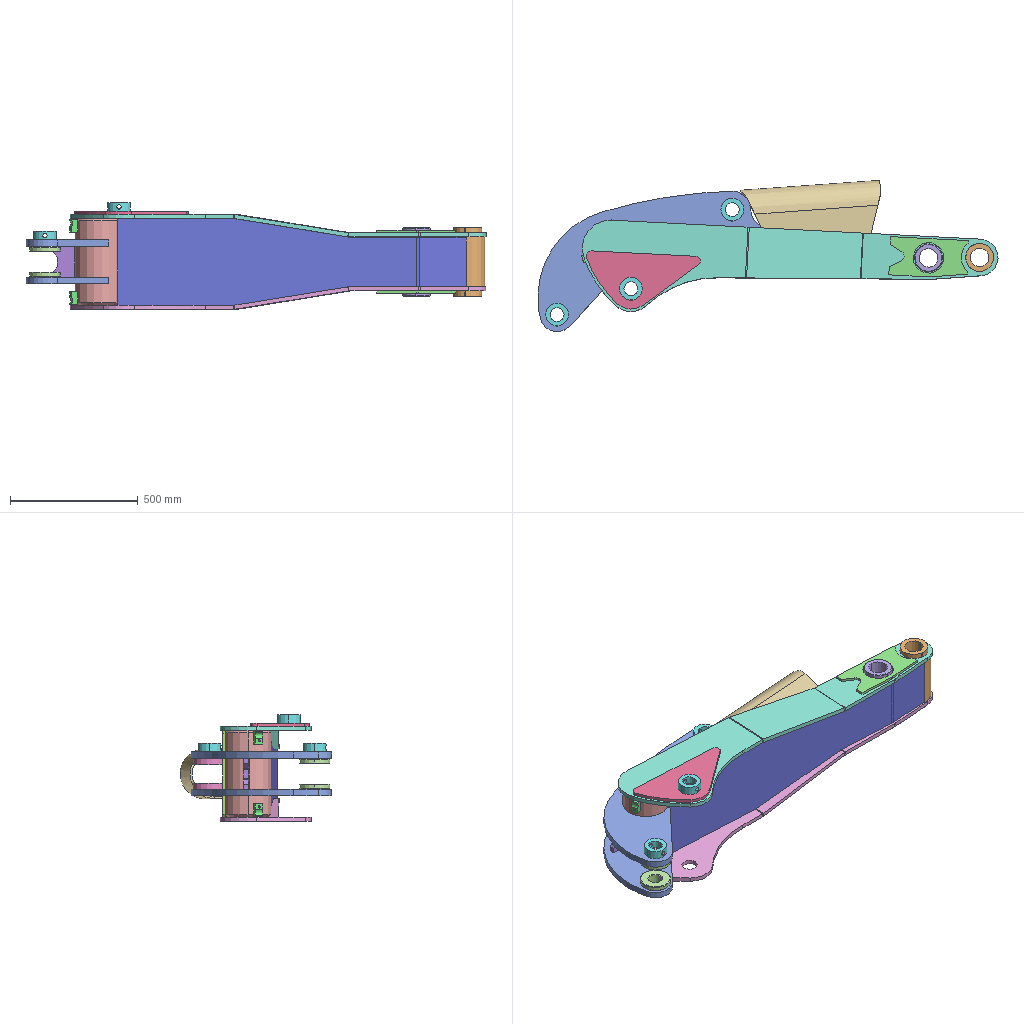Assembly | SolidWorks | 21 different items | 28 placed | box 1804 x 593 x 419 mm
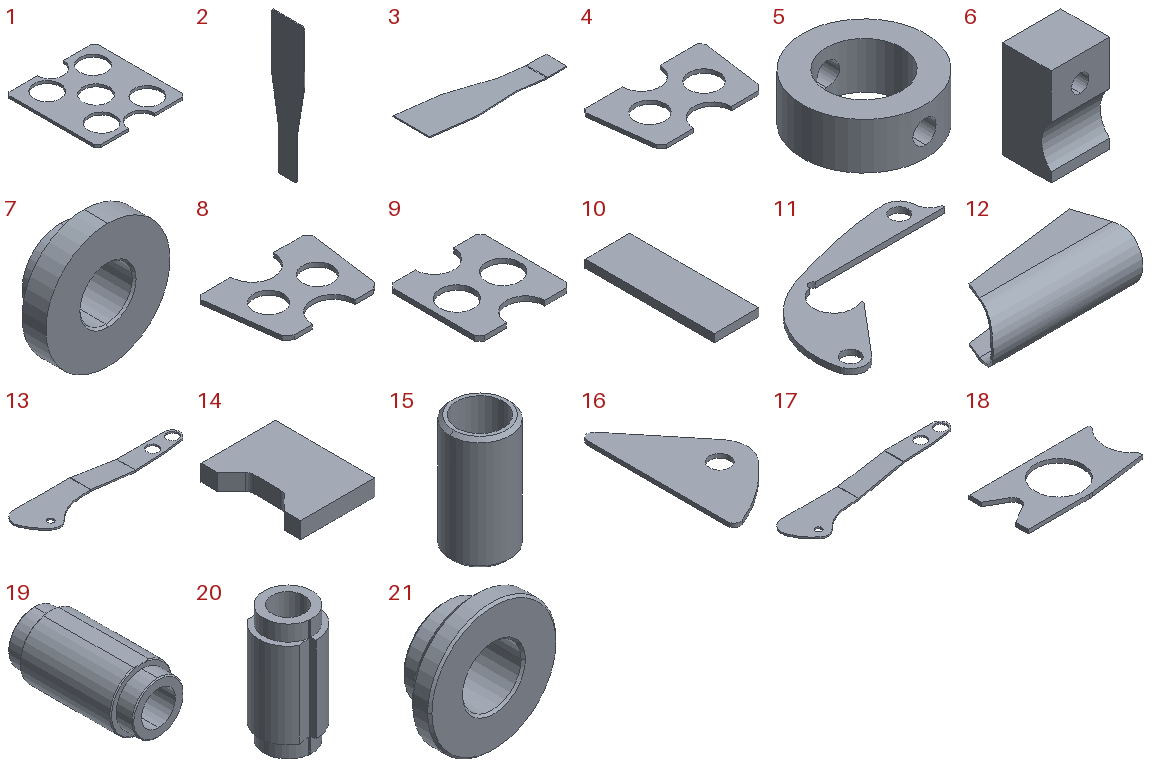Parts list (item | quantity | size | volume | features):
1 | x1 | 340 x 350 x 10 mm | 715881 mm3 | features Extrusion 1
2 | x1 | 10 x 340 x 1438 mm | 3900020 mm3 | features Extrusion 1
3 | x1 | 1360 x 340 x 153.769 mm | 3656500 mm3 | features FlatPattern 1, SM3dBend 1, SMBaseFlange 1, SheetMetal 1
4 | x1 | 316.869 x 190 x 10 mm | 378498 mm3 | features Extrusion 1
5 | x3 | 90 x 90 x 34 mm | 127515 mm3 | features Extrusion 1, ICE 1
6 | x2 | 30 x 25 x 50 mm | 33718 mm3 | features Extrusion 1, HoleWzd 1, ICE 1
7 | x2 | 130 x 50 x 130 mm | 338349 mm3 | features Revolution 1
8 | x1 | 260.209 x 190 x 10 mm | 293760 mm3 | features Extrusion 1
9 | x1 | 192 x 190 x 10 mm | 235565 mm3 | features Extrusion 1
10 | x1 | 68 x 195 x 12 mm | 159120 mm3 | features Extrusion 1
11 | x2 | 873.891 x 585.5 x 25 mm | 3320222 mm3 | features Extrusion 1
12 | x1 | 545.7 x 215.495 x 196 mm | 1900724 mm3 | features FlatPattern 1, SM3dBend 1, SMBaseFlange 1, SheetMetal 1
13 | x1 | 1631 x 354.5 x 88.747 mm | 5017835 mm3 | features SM3dBend 2, FlatPattern 1, SMBaseFlange 1, SheetMetal 1
14 | x1 | 90 x 121 x 20 mm | 193486 mm3 | features Extrusion 1
15 | x1 | 180 x 180 x 341 mm | 3373652 mm3 | features Chamfer 1, Extrusion 1
16 | x1 | 220 x 447.752 x 12 mm | 720833 mm3 | features Extrusion 1
17 | x1 | 1631 x 354.5 x 88.747 mm | 5017835 mm3 | features SM3dBend 2, FlatPattern 1, SMBaseFlange 1, SheetMetal 1
18 | x2 | 309.8 x 150 x 10 mm | 282199 mm3 | features Extrusion 1
19 | x1 | 133 x 268 x 129 mm | 2265782 mm3 | features ICE 1, Revolution 1
20 | x1 | 133 x 133 x 268 mm | 2196545 mm3 | features ICE 2, Extrusion 1
21 | x2 | 120 x 46 x 120 mm | 247351 mm3 | features Revolution 1
Mates (type | each side: item.copy, entity, surface, feature):
Concentric | 15.1 face cylinder Boss-Extrude1 | 11.1 face cylinder Boss-Extrude1
DistanceDim | 11.2 face plane Boss-Extrude1 | 11.1 face plane Boss-Extrude1
Coincident | 11.1 face plane Boss-Extrude1 | 2.1 face plane Boss-Extrude1
Parallel | 11.2 edge | 2.1 face plane Boss-Extrude1
Coincident | 15.1 face plane Boss-Extrude1 | 17.1 face plane Base-Flange1
Concentric | 15.1 face cylinder Boss-Extrude1 | 17.1 edge
Coincident | 2.1 face plane Boss-Extrude1 | 17.1 face plane Base-Flange1
Parallel | 2.1 face plane Boss-Extrude1 | 17.1 face plane Base-Flange1
Concentric | 15.1 face cylinder Boss-Extrude1 | 13.1 edge
Coincident | 15.1 face plane Boss-Extrude1 | 13.1 face plane Base-Flange1
Parallel | 2.1 face plane Boss-Extrude1 | 13.1 face plane Base-Flange1
Concentric | 13.1 face cylinder Base-Flange1 | 20.1 face cylinder Cut-Extrude1
Coincident | 13.1 face plane Sketched Bend7 | 20.1 face plane Cut-Extrude1
Coincident | 2.1 face plane Boss-Extrude1 | 20.1 face plane Boss-Extrude1
Concentric | 13.1 face cylinder Base-Flange1 | 19.1 face cylinder Revolve1
Coincident | 13.1 face plane Sketched Bend7 | 19.1 face plane Revolve1
Parallel | 2.1 face plane Boss-Extrude1 | 19.1 face plane Cut-Extrude1
Concentric | 19.1 face cylinder Revolve1 | 18.1 face cylinder Boss-Extrude1
Coincident | 13.1 face plane Sketched Bend7 | 18.1 face plane Boss-Extrude1
Concentric | 20.1 face cylinder Boss-Extrude1 | 18.1 face cylinder Boss-Extrude1
Concentric | 13.1 face cylinder Base-Flange1 | 16.1 face cylinder Boss-Extrude1
Coincident | 13.1 face plane Base-Flange1 | 16.1 face plane Boss-Extrude1
Parallel | 13.1 face plane Base-Flange1 | 16.1 face plane Boss-Extrude1
DistanceDim | 13.1 face plane Base-Flange1 | 1.1 face plane Boss-Extrude1
PlanarAngleDim | 1.1 face plane Boss-Extrude1 | 2.1 face plane Boss-Extrude1
Coincident | 2.1 face plane Boss-Extrude1 | 1.1 edge
Coincident | 15.1 face cylinder Boss-Extrude1 | 1.1 edge
PlanarAngleDim | 4.1 face plane Boss-Extrude1 | 2.1 face plane Boss-Extrude1
Coincident | 2.1 face plane Boss-Extrude1 | 4.1 edge
DistanceDim | 4.1 edge | 1.1 edge
PlanarAngleDim | 8.1 face plane Boss-Extrude1 | 2.1 face plane Boss-Extrude1
Coincident | 2.1 face plane Boss-Extrude1 | 8.1 edge
DistanceDim | 8.1 edge | 20.1 edge
Coincident | 13.1 face plane Sketched Bend6 | 4.1 vertex
Coincident | 13.1 face plane Sketched Bend6 | 8.1 vertex
DistanceDim | 20.1 edge | 9.1 edge
Coincident | 2.1 face plane Boss-Extrude1 | 9.1 edge
PlanarAngleDim | 9.1 face plane Boss-Extrude1 | 2.1 face plane Boss-Extrude1
DistanceDim | 9.1 edge | 17.1 face plane Sketched Bend7
Coincident | 17.1 face plane Sketched Bend7 | 10.1 face plane Boss-Extrude1
DistanceDim | 2.1 face plane Boss-Extrude1 | 10.1 face plane Boss-Extrude1
Coincident | 20.1 face cylinder Boss-Extrude1 | 10.1 edge
Parallel | 2.1 face plane Boss-Extrude1 | 3.1 face plane Sketched Bend1
Coincident | 20.1 edge | 3.1 edge
DistanceDim | 13.1 face plane Sketched Bend7 | 3.1 face plane Base-Flange1
Concentric | 11.1 face cylinder Boss-Extrude1 | 21.1 face cylinder Revolve1
Coincident | 11.1 face plane Boss-Extrude1 | 21.1 face plane Revolve1
Concentric | 11.2 face cylinder Boss-Extrude1 | 21.2 face cylinder Revolve1
Coincident | 11.2 face plane Boss-Extrude1 | 21.2 face plane Revolve1
Concentric | 11.1 face cylinder Boss-Extrude1 | 7.1 face cylinder Revolve1
Coincident | 11.1 face plane Boss-Extrude1 | 7.1 face plane Revolve1
Concentric | 11.2 face cylinder Boss-Extrude1 | 7.2 face cylinder Revolve1
Coincident | 11.2 face plane Boss-Extrude1 | 7.2 face plane Revolve1
Concentric | 7.1 face cylinder Revolve1 | 5.1 face cylinder Boss-Extrude1
Coincident | 11.1 face plane Boss-Extrude1 | 5.1 face plane Boss-Extrude1
Concentric | 16.1 face cylinder Boss-Extrude1 | 5.2 face cylinder Boss-Extrude1
Coincident | 16.1 face plane Boss-Extrude1 | 5.2 face plane Boss-Extrude1
Concentric | 21.1 face cylinder Revolve1 | 5.3 face cylinder Boss-Extrude1
Coincident | 11.1 face plane Boss-Extrude1 | 5.3 face plane Boss-Extrude1
Coincident | 2.1 face plane Boss-Extrude1 | 12.1 face plane Base-Flange1
Parallel | 13.1 face plane Sketched Bend7 | 12.1 face plane Base-Flange1
Coincident | 17.1 face plane Sketched Bend7 | 12.1 face plane Sketched Bend2
Parallel | 2.1 face plane Boss-Extrude1 | 14.1 face plane Boss-Extrude1
Coincident | 11.2 face plane Boss-Extrude1 | 14.1 face plane Boss-Extrude1
Tangent | 15.1 face cylinder Boss-Extrude1 | 14.1 face plane Boss-Extrude1
DistanceDim | 2.1 face plane Boss-Extrude1 | 14.1 face plane Boss-Extrude1
DistanceDim | 6.1 face plane Boss-Extrude1 | 17.1 face plane Base-Flange1
Tangent | 15.1 face cylinder Boss-Extrude1 | 6.1 face plane Boss-Extrude1
DistanceDim | 2.1 face plane Boss-Extrude1 | 6.1 edge
Tangent | 11.2 face cylinder Boss-Extrude1 | 12.1 face plane Base-Flange1